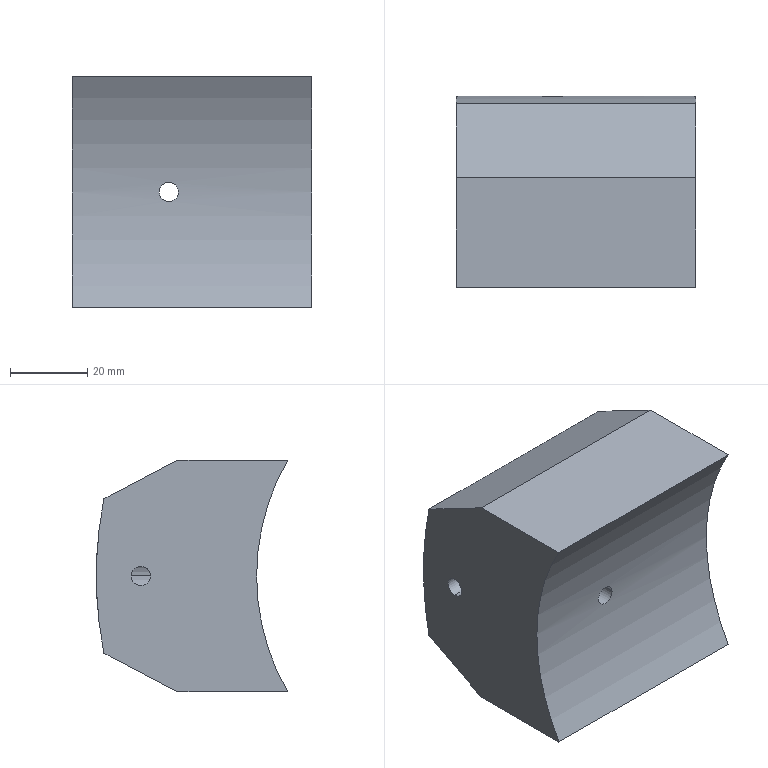Part | STEP file | Input 14 | 1 solid | 19 faces | box 62 x 49.538 x 60 mm | volume 146146 mm3 | cylinder 10 | plane 7 | cone 2 | commonest cylinder face diameters 5 x4 8.5 x2 10 x2 120 x1 203 x1